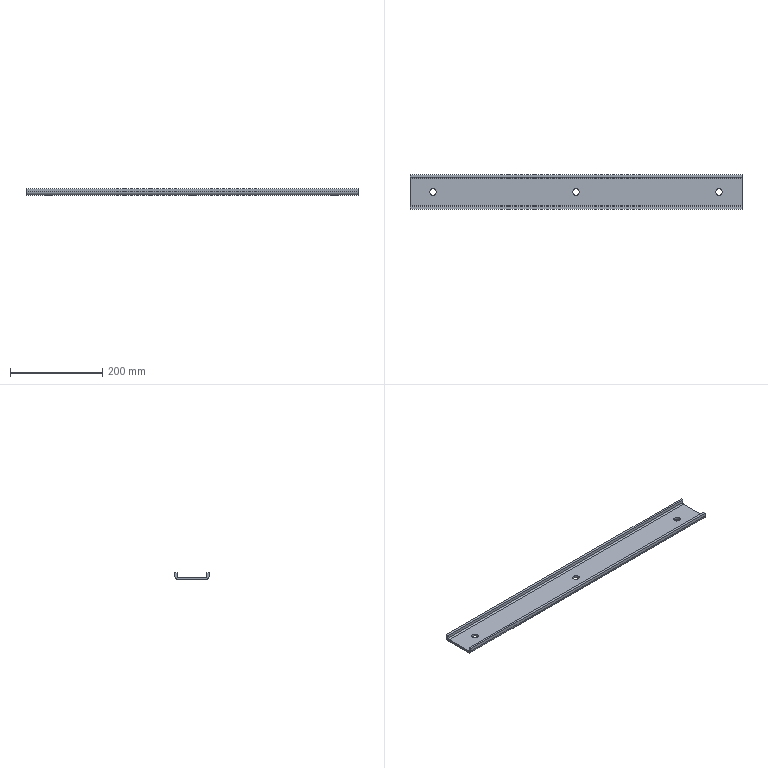Part | SolidWorks | features MoveFace 4, Fillet 2, BaseBody 1, ICE 1 | 1 solid | 20 faces | box 720 x 75 x 15 mm | volume 322694 mm3 | cylinder 10 | plane 10 | commonest cylinder face diameters 14 x6 6 x2 16 x2
STEP:
#1=CARTESIAN_POINT('',(-7.,0.,0.));
#2=VERTEX_POINT('',#1);
#3=CARTESIAN_POINT('',(7.,0.,0.));
#4=VERTEX_POINT('',#3);
#5=CARTESIAN_POINT('',(0.,0.,0.));
#6=DIRECTION('',(0.,0.,1.));
#7=DIRECTION('',(1.,0.,0.));
#8=AXIS2_PLACEMENT_3D('',#5,#6,#7);
#9=CIRCLE('',#8,7.);
#10=EDGE_CURVE('',#2,#4,#9,.T.);
#11=ORIENTED_EDGE('',*,*,#10,.F.);
#12=CARTESIAN_POINT('',(-7.,0.,5.));
#13=VERTEX_POINT('',#12);
#14=CARTESIAN_POINT('',(-7.,0.,-5.));
#15=DIRECTION('',(0.,0.,1.));
#16=VECTOR('',#15,1000.);
#17=LINE('',#14,#16);
#18=EDGE_CURVE('',#2,#13,#17,.T.);
#19=ORIENTED_EDGE('',*,*,#18,.T.);
#20=CARTESIAN_POINT('',(7.,0.,5.));
#21=VERTEX_POINT('',#20);
#22=CARTESIAN_POINT('',(0.,0.,5.));
#23=DIRECTION('',(0.,0.,-1.));
#24=DIRECTION('',(1.,0.,0.));
#25=AXIS2_PLACEMENT_3D('',#22,#23,#24);
#26=CIRCLE('',#25,7.);
#27=EDGE_CURVE('',#21,#13,#26,.T.);
#28=ORIENTED_EDGE('',*,*,#27,.F.);
#29=CARTESIAN_POINT('',(7.,0.,-5.));
#30=DIRECTION('',(0.,0.,1.));
#31=VECTOR('',#30,1000.);
#32=LINE('',#29,#31);
#33=EDGE_CURVE('',#4,#21,#32,.T.);
#34=ORIENTED_EDGE('',*,*,#33,.F.);
#35=EDGE_LOOP('',(#11,#19,#28,#34));
#36=FACE_OUTER_BOUND('',#35,.T.);
#37=CARTESIAN_POINT('',(0.,0.,-5.));
#38=DIRECTION('',(0.,0.,1.));
#39=DIRECTION('',(1.,0.,0.));
#40=AXIS2_PLACEMENT_3D('',#37,#38,#39);
#41=CYLINDRICAL_SURFACE('',#40,7.);
#42=ADVANCED_FACE('',(#36),#41,.F.);
#43=CARTESIAN_POINT('',(-317.,0.,0.));
#44=VERTEX_POINT('',#43);
#45=CARTESIAN_POINT('',(-303.,0.,0.));
#46=VERTEX_POINT('',#45);
#47=CARTESIAN_POINT('',(-310.,0.,0.));
#48=DIRECTION('',(0.,0.,1.));
#49=DIRECTION('',(1.,0.,0.));
#50=AXIS2_PLACEMENT_3D('',#47,#48,#49);
#51=CIRCLE('',#50,7.);
#52=EDGE_CURVE('',#44,#46,#51,.T.);
#53=ORIENTED_EDGE('',*,*,#52,.F.);
#54=CARTESIAN_POINT('',(-317.,0.,5.));
#55=VERTEX_POINT('',#54);
#56=CARTESIAN_POINT('',(-317.,0.,-5.));
#57=DIRECTION('',(0.,0.,1.));
#58=VECTOR('',#57,1000.);
#59=LINE('',#56,#58);
#60=EDGE_CURVE('',#44,#55,#59,.T.);
#61=ORIENTED_EDGE('',*,*,#60,.T.);
#62=CARTESIAN_POINT('',(-303.,0.,5.));
#63=VERTEX_POINT('',#62);
#64=CARTESIAN_POINT('',(-310.,0.,5.));
#65=DIRECTION('',(0.,0.,-1.));
#66=DIRECTION('',(1.,0.,0.));
#67=AXIS2_PLACEMENT_3D('',#64,#65,#66);
#68=CIRCLE('',#67,7.);
#69=EDGE_CURVE('',#63,#55,#68,.T.);
#70=ORIENTED_EDGE('',*,*,#69,.F.);
#71=CARTESIAN_POINT('',(-303.,0.,-5.));
#72=DIRECTION('',(0.,0.,1.));
#73=VECTOR('',#72,1000.);
#74=LINE('',#71,#73);
#75=EDGE_CURVE('',#46,#63,#74,.T.);
#76=ORIENTED_EDGE('',*,*,#75,.F.);
#77=EDGE_LOOP('',(#53,#61,#70,#76));
#78=FACE_OUTER_BOUND('',#77,.T.);
#79=CARTESIAN_POINT('',(-310.,0.,-5.));
#80=DIRECTION('',(0.,0.,1.));
#81=DIRECTION('',(1.,0.,0.));
#82=AXIS2_PLACEMENT_3D('',#79,#80,#81);
#83=CYLINDRICAL_SURFACE('',#82,7.);
#84=ADVANCED_FACE('',(#78),#83,.F.);
#85=CARTESIAN_POINT('',(303.,0.,0.));
#86=VERTEX_POINT('',#85);
#87=CARTESIAN_POINT('',(317.,0.,0.));
#88=VERTEX_POINT('',#87);
#89=CARTESIAN_POINT('',(310.,0.,0.));
#90=DIRECTION('',(0.,0.,1.));
#91=DIRECTION('',(1.,0.,0.));
#92=AXIS2_PLACEMENT_3D('',#89,#90,#91);
#93=CIRCLE('',#92,7.);
#94=EDGE_CURVE('',#86,#88,#93,.T.);
#95=ORIENTED_EDGE('',*,*,#94,.F.);
#96=CARTESIAN_POINT('',(303.,0.,5.));
#97=VERTEX_POINT('',#96);
#98=CARTESIAN_POINT('',(303.,0.,-5.));
#99=DIRECTION('',(0.,0.,1.));
#100=VECTOR('',#99,1000.);
#101=LINE('',#98,#100);
#102=EDGE_CURVE('',#86,#97,#101,.T.);
#103=ORIENTED_EDGE('',*,*,#102,.T.);
#104=CARTESIAN_POINT('',(317.,0.,5.));
#105=VERTEX_POINT('',#104);
#106=CARTESIAN_POINT('',(310.,0.,5.));
#107=DIRECTION('',(0.,0.,-1.));
#108=DIRECTION('',(1.,0.,0.));
#109=AXIS2_PLACEMENT_3D('',#106,#107,#108);
#110=CIRCLE('',#109,7.);
#111=EDGE_CURVE('',#105,#97,#110,.T.);
#112=ORIENTED_EDGE('',*,*,#111,.F.);
#113=CARTESIAN_POINT('',(317.,0.,-5.));
#114=DIRECTION('',(0.,0.,1.));
#115=VECTOR('',#114,1000.);
#116=LINE('',#113,#115);
#117=EDGE_CURVE('',#88,#105,#116,.T.);
#118=ORIENTED_EDGE('',*,*,#117,.F.);
#119=EDGE_LOOP('',(#95,#103,#112,#118));
#120=FACE_OUTER_BOUND('',#119,.T.);
#121=CARTESIAN_POINT('',(310.,0.,-5.));
#122=DIRECTION('',(0.,0.,1.));
#123=DIRECTION('',(1.,0.,0.));
#124=AXIS2_PLACEMENT_3D('',#121,#122,#123);
#125=CYLINDRICAL_SURFACE('',#124,7.);
#126=ADVANCED_FACE('',(#120),#125,.F.);
#127=ORIENTED_EDGE('',*,*,#27,.T.);
#128=CARTESIAN_POINT('',(0.,0.,5.));
#129=DIRECTION('',(0.,0.,-1.));
#130=DIRECTION('',(1.,0.,0.));
#131=AXIS2_PLACEMENT_3D('',#128,#129,#130);
#132=CIRCLE('',#131,7.);
#133=EDGE_CURVE('',#13,#21,#132,.T.);
#134=ORIENTED_EDGE('',*,*,#133,.T.);
#135=EDGE_LOOP('',(#127,#134));
#136=FACE_BOUND('',#135,.T.);
#137=ORIENTED_EDGE('',*,*,#69,.T.);
#138=CARTESIAN_POINT('',(-310.,0.,5.));
#139=DIRECTION('',(0.,0.,-1.));
#140=DIRECTION('',(1.,0.,0.));
#141=AXIS2_PLACEMENT_3D('',#138,#139,#140);
#142=CIRCLE('',#141,7.);
#143=EDGE_CURVE('',#55,#63,#142,.T.);
#144=ORIENTED_EDGE('',*,*,#143,.T.);
#145=EDGE_LOOP('',(#137,#144));
#146=FACE_BOUND('',#145,.T.);
#147=ORIENTED_EDGE('',*,*,#111,.T.);
#148=CARTESIAN_POINT('',(310.,0.,5.));
#149=DIRECTION('',(0.,0.,-1.));
#150=DIRECTION('',(1.,0.,0.));
#151=AXIS2_PLACEMENT_3D('',#148,#149,#150);
#152=CIRCLE('',#151,7.);
#153=EDGE_CURVE('',#97,#105,#152,.T.);
#154=ORIENTED_EDGE('',*,*,#153,.T.);
#155=EDGE_LOOP('',(#147,#154));
#156=FACE_BOUND('',#155,.T.);
#157=CARTESIAN_POINT('',(-360.,29.5,5.));
#158=VERTEX_POINT('',#157);
#159=CARTESIAN_POINT('',(-360.,-29.5,5.));
#160=VERTEX_POINT('',#159);
#161=CARTESIAN_POINT('',(-360.,0.,5.));
#162=DIRECTION('',(0.,-1.,0.));
#163=VECTOR('',#162,1000.);
#164=LINE('',#161,#163);
#165=EDGE_CURVE('',#158,#160,#164,.T.);
#166=ORIENTED_EDGE('',*,*,#165,.T.);
#167=CARTESIAN_POINT('',(360.,-29.5,5.));
#168=VERTEX_POINT('',#167);
#169=CARTESIAN_POINT('',(0.,-29.5,5.));
#170=DIRECTION('',(1.,0.,0.));
#171=VECTOR('',#170,1000.);
#172=LINE('',#169,#171);
#173=EDGE_CURVE('',#160,#168,#172,.T.);
#174=ORIENTED_EDGE('',*,*,#173,.T.);
#175=CARTESIAN_POINT('',(360.,29.5,5.));
#176=VERTEX_POINT('',#175);
#177=CARTESIAN_POINT('',(360.,0.,5.));
#178=DIRECTION('',(0.,1.,0.));
#179=VECTOR('',#178,1000.);
#180=LINE('',#177,#179);
#181=EDGE_CURVE('',#168,#176,#180,.T.);
#182=ORIENTED_EDGE('',*,*,#181,.T.);
#183=CARTESIAN_POINT('',(0.,29.5,5.));
#184=DIRECTION('',(-1.,0.,0.));
#185=VECTOR('',#184,1000.);
#186=LINE('',#183,#185);
#187=EDGE_CURVE('',#176,#158,#186,.T.);
#188=ORIENTED_EDGE('',*,*,#187,.T.);
#189=EDGE_LOOP('',(#166,#174,#182,#188));
#190=FACE_OUTER_BOUND('',#189,.T.);
#191=CARTESIAN_POINT('',(0.,0.,5.));
#192=DIRECTION('',(0.,0.,1.));
#193=DIRECTION('',(1.,0.,0.));
#194=AXIS2_PLACEMENT_3D('',#191,#192,#193);
#195=PLANE('',#194);
#196=ADVANCED_FACE('',(#136,#146,#156,#190),#195,.T.);
#197=CARTESIAN_POINT('',(-360.,-37.5,8.));
#198=VERTEX_POINT('',#197);
#199=CARTESIAN_POINT('',(-360.,-37.5,15.));
#200=VERTEX_POINT('',#199);
#201=CARTESIAN_POINT('',(-360.,-37.5,5.));
#202=DIRECTION('',(0.,0.,1.));
#203=VECTOR('',#202,1000.);
#204=LINE('',#201,#203);
#205=EDGE_CURVE('',#198,#200,#204,.T.);
#206=ORIENTED_EDGE('',*,*,#205,.F.);
#207=CARTESIAN_POINT('',(360.,-37.5,8.));
#208=VERTEX_POINT('',#207);
#209=CARTESIAN_POINT('',(-360.,-37.5,8.));
#210=DIRECTION('',(1.,0.,0.));
#211=VECTOR('',#210,1000.);
#212=LINE('',#209,#211);
#213=EDGE_CURVE('',#198,#208,#212,.T.);
#214=ORIENTED_EDGE('',*,*,#213,.T.);
#215=CARTESIAN_POINT('',(360.,-37.5,15.));
#216=VERTEX_POINT('',#215);
#217=CARTESIAN_POINT('',(360.,-37.5,5.));
#218=DIRECTION('',(0.,0.,-1.));
#219=VECTOR('',#218,1000.);
#220=LINE('',#217,#219);
#221=EDGE_CURVE('',#216,#208,#220,.T.);
#222=ORIENTED_EDGE('',*,*,#221,.F.);
#223=CARTESIAN_POINT('',(-300.,-37.5,15.));
#224=DIRECTION('',(1.,0.,0.));
#225=VECTOR('',#224,1000.);
#226=LINE('',#223,#225);
#227=EDGE_CURVE('',#200,#216,#226,.T.);
#228=ORIENTED_EDGE('',*,*,#227,.F.);
#229=EDGE_LOOP('',(#206,#214,#222,#228));
#230=FACE_OUTER_BOUND('',#229,.T.);
#231=CARTESIAN_POINT('',(-360.,-37.5,5.));
#232=DIRECTION('',(0.,1.,0.));
#233=DIRECTION('',(0.,0.,1.));
#234=AXIS2_PLACEMENT_3D('',#231,#232,#233);
#235=PLANE('',#234);
#236=ADVANCED_FACE('',(#230),#235,.F.);
#237=CARTESIAN_POINT('',(-360.,-29.5,0.));
#238=VERTEX_POINT('',#237);
#239=CARTESIAN_POINT('',(-360.,29.5,0.));
#240=VERTEX_POINT('',#239);
#241=CARTESIAN_POINT('',(-360.,37.5,0.));
#242=DIRECTION('',(0.,1.,0.));
#243=VECTOR('',#242,1000.);
#244=LINE('',#241,#243);
#245=EDGE_CURVE('',#238,#240,#244,.T.);
#246=ORIENTED_EDGE('',*,*,#245,.F.);
#247=CARTESIAN_POINT('',(-360.,-29.5,8.));
#248=DIRECTION('',(-1.,0.,0.));
#249=DIRECTION('',(0.,0.,-1.));
#250=AXIS2_PLACEMENT_3D('',#247,#248,#249);
#251=CIRCLE('',#250,8.);
#252=EDGE_CURVE('',#238,#198,#251,.T.);
#253=ORIENTED_EDGE('',*,*,#252,.T.);
#254=ORIENTED_EDGE('',*,*,#205,.T.);
#255=CARTESIAN_POINT('',(-360.,-32.5,15.));
#256=VERTEX_POINT('',#255);
#257=CARTESIAN_POINT('',(-360.,-37.5,15.));
#258=DIRECTION('',(0.,-1.,0.));
#259=VECTOR('',#258,1000.);
#260=LINE('',#257,#259);
#261=EDGE_CURVE('',#256,#200,#260,.T.);
#262=ORIENTED_EDGE('',*,*,#261,.F.);
#263=CARTESIAN_POINT('',(-360.,-32.5,8.));
#264=VERTEX_POINT('',#263);
#265=CARTESIAN_POINT('',(-360.,-32.5,15.));
#266=DIRECTION('',(0.,0.,-1.));
#267=VECTOR('',#266,1000.);
#268=LINE('',#265,#267);
#269=EDGE_CURVE('',#256,#264,#268,.T.);
#270=ORIENTED_EDGE('',*,*,#269,.T.);
#271=CARTESIAN_POINT('',(-360.,-29.5,8.));
#272=DIRECTION('',(1.,0.,0.));
#273=DIRECTION('',(0.,0.,-1.));
#274=AXIS2_PLACEMENT_3D('',#271,#272,#273);
#275=CIRCLE('',#274,3.);
#276=EDGE_CURVE('',#264,#160,#275,.T.);
#277=ORIENTED_EDGE('',*,*,#276,.T.);
#278=ORIENTED_EDGE('',*,*,#165,.F.);
#279=CARTESIAN_POINT('',(-360.,32.5,8.));
#280=VERTEX_POINT('',#279);
#281=CARTESIAN_POINT('',(-360.,29.5,8.));
#282=DIRECTION('',(1.,0.,0.));
#283=DIRECTION('',(0.,0.,-1.));
#284=AXIS2_PLACEMENT_3D('',#281,#282,#283);
#285=CIRCLE('',#284,3.);
#286=EDGE_CURVE('',#158,#280,#285,.T.);
#287=ORIENTED_EDGE('',*,*,#286,.T.);
#288=CARTESIAN_POINT('',(-360.,32.5,15.));
#289=VERTEX_POINT('',#288);
#290=CARTESIAN_POINT('',(-360.,32.5,15.));
#291=DIRECTION('',(0.,0.,-1.));
#292=VECTOR('',#291,1000.);
#293=LINE('',#290,#292);
#294=EDGE_CURVE('',#289,#280,#293,.T.);
#295=ORIENTED_EDGE('',*,*,#294,.F.);
#296=CARTESIAN_POINT('',(-360.,37.5,15.));
#297=VERTEX_POINT('',#296);
#298=CARTESIAN_POINT('',(-360.,37.5,15.));
#299=DIRECTION('',(0.,-1.,0.));
#300=VECTOR('',#299,1000.);
#301=LINE('',#298,#300);
#302=EDGE_CURVE('',#297,#289,#301,.T.);
#303=ORIENTED_EDGE('',*,*,#302,.F.);
#304=CARTESIAN_POINT('',(-360.,37.5,8.));
#305=VERTEX_POINT('',#304);
#306=CARTESIAN_POINT('',(-360.,37.5,5.));
#307=DIRECTION('',(0.,0.,1.));
#308=VECTOR('',#307,1000.);
#309=LINE('',#306,#308);
#310=EDGE_CURVE('',#305,#297,#309,.T.);
#311=ORIENTED_EDGE('',*,*,#310,.F.);
#312=CARTESIAN_POINT('',(-360.,29.5,8.));
#313=DIRECTION('',(-1.,0.,0.));
#314=DIRECTION('',(0.,0.,-1.));
#315=AXIS2_PLACEMENT_3D('',#312,#313,#314);
#316=CIRCLE('',#315,8.);
#317=EDGE_CURVE('',#305,#240,#316,.T.);
#318=ORIENTED_EDGE('',*,*,#317,.T.);
#319=EDGE_LOOP('',(#246,#253,#254,#262,#270,#277,#278,#287,#295,#303,#311,#318));
#320=FACE_OUTER_BOUND('',#319,.T.);
#321=CARTESIAN_POINT('',(-360.,37.5,5.));
#322=DIRECTION('',(1.,0.,0.));
#323=DIRECTION('',(0.,0.,-1.));
#324=AXIS2_PLACEMENT_3D('',#321,#322,#323);
#325=PLANE('',#324);
#326=ADVANCED_FACE('',(#320),#325,.F.);
#327=CARTESIAN_POINT('',(360.,37.5,8.));
#328=VERTEX_POINT('',#327);
#329=CARTESIAN_POINT('',(360.,37.5,15.));
#330=VERTEX_POINT('',#329);
#331=CARTESIAN_POINT('',(360.,37.5,5.));
#332=DIRECTION('',(0.,0.,1.));
#333=VECTOR('',#332,1000.);
#334=LINE('',#331,#333);
#335=EDGE_CURVE('',#328,#330,#334,.T.);
#336=ORIENTED_EDGE('',*,*,#335,.F.);
#337=CARTESIAN_POINT('',(-360.,37.5,8.));
#338=DIRECTION('',(-1.,0.,0.));
#339=VECTOR('',#338,1000.);
#340=LINE('',#337,#339);
#341=EDGE_CURVE('',#328,#305,#340,.T.);
#342=ORIENTED_EDGE('',*,*,#341,.T.);
#343=ORIENTED_EDGE('',*,*,#310,.T.);
#344=CARTESIAN_POINT('',(-300.,37.5,15.));
#345=DIRECTION('',(-1.,0.,0.));
#346=VECTOR('',#345,1000.);
#347=LINE('',#344,#346);
#348=EDGE_CURVE('',#330,#297,#347,.T.);
#349=ORIENTED_EDGE('',*,*,#348,.F.);
#350=EDGE_LOOP('',(#336,#342,#343,#349));
#351=FACE_OUTER_BOUND('',#350,.T.);
#352=CARTESIAN_POINT('',(-360.,37.5,5.));
#353=DIRECTION('',(0.,-1.,0.));
#354=DIRECTION('',(0.,0.,-1.));
#355=AXIS2_PLACEMENT_3D('',#352,#353,#354);
#356=PLANE('',#355);
#357=ADVANCED_FACE('',(#351),#356,.F.);
#358=ORIENTED_EDGE('',*,*,#221,.T.);
#359=CARTESIAN_POINT('',(360.,-29.5,0.));
#360=VERTEX_POINT('',#359);
#361=CARTESIAN_POINT('',(360.,-29.5,8.));
#362=DIRECTION('',(1.,0.,0.));
#363=DIRECTION('',(0.,0.,1.));
#364=AXIS2_PLACEMENT_3D('',#361,#362,#363);
#365=CIRCLE('',#364,8.);
#366=EDGE_CURVE('',#208,#360,#365,.T.);
#367=ORIENTED_EDGE('',*,*,#366,.T.);
#368=CARTESIAN_POINT('',(360.,29.5,0.));
#369=VERTEX_POINT('',#368);
#370=CARTESIAN_POINT('',(360.,37.5,0.));
#371=DIRECTION('',(0.,-1.,0.));
#372=VECTOR('',#371,1000.);
#373=LINE('',#370,#372);
#374=EDGE_CURVE('',#369,#360,#373,.T.);
#375=ORIENTED_EDGE('',*,*,#374,.F.);
#376=CARTESIAN_POINT('',(360.,29.5,8.));
#377=DIRECTION('',(1.,0.,0.));
#378=DIRECTION('',(0.,0.,1.));
#379=AXIS2_PLACEMENT_3D('',#376,#377,#378);
#380=CIRCLE('',#379,8.);
#381=EDGE_CURVE('',#369,#328,#380,.T.);
#382=ORIENTED_EDGE('',*,*,#381,.T.);
#383=ORIENTED_EDGE('',*,*,#335,.T.);
#384=CARTESIAN_POINT('',(360.,32.5,15.));
#385=VERTEX_POINT('',#384);
#386=CARTESIAN_POINT('',(360.,37.5,15.));
#387=DIRECTION('',(0.,1.,0.));
#388=VECTOR('',#387,1000.);
#389=LINE('',#386,#388);
#390=EDGE_CURVE('',#385,#330,#389,.T.);
#391=ORIENTED_EDGE('',*,*,#390,.F.);
#392=CARTESIAN_POINT('',(360.,32.5,8.));
#393=VERTEX_POINT('',#392);
#394=CARTESIAN_POINT('',(360.,32.5,15.));
#395=DIRECTION('',(0.,0.,-1.));
#396=VECTOR('',#395,1000.);
#397=LINE('',#394,#396);
#398=EDGE_CURVE('',#385,#393,#397,.T.);
#399=ORIENTED_EDGE('',*,*,#398,.T.);
#400=CARTESIAN_POINT('',(360.,29.5,8.));
#401=DIRECTION('',(-1.,0.,0.));
#402=DIRECTION('',(0.,0.,1.));
#403=AXIS2_PLACEMENT_3D('',#400,#401,#402);
#404=CIRCLE('',#403,3.);
#405=EDGE_CURVE('',#393,#176,#404,.T.);
#406=ORIENTED_EDGE('',*,*,#405,.T.);
#407=ORIENTED_EDGE('',*,*,#181,.F.);
#408=CARTESIAN_POINT('',(360.,-32.5,8.));
#409=VERTEX_POINT('',#408);
#410=CARTESIAN_POINT('',(360.,-29.5,8.));
#411=DIRECTION('',(-1.,0.,0.));
#412=DIRECTION('',(0.,0.,1.));
#413=AXIS2_PLACEMENT_3D('',#410,#411,#412);
#414=CIRCLE('',#413,3.);
#415=EDGE_CURVE('',#168,#409,#414,.T.);
#416=ORIENTED_EDGE('',*,*,#415,.T.);
#417=CARTESIAN_POINT('',(360.,-32.5,15.));
#418=VERTEX_POINT('',#417);
#419=CARTESIAN_POINT('',(360.,-32.5,15.));
#420=DIRECTION('',(0.,0.,-1.));
#421=VECTOR('',#420,1000.);
#422=LINE('',#419,#421);
#423=EDGE_CURVE('',#418,#409,#422,.T.);
#424=ORIENTED_EDGE('',*,*,#423,.F.);
#425=CARTESIAN_POINT('',(360.,-37.5,15.));
#426=DIRECTION('',(0.,1.,0.));
#427=VECTOR('',#426,1000.);
#428=LINE('',#425,#427);
#429=EDGE_CURVE('',#216,#418,#428,.T.);
#430=ORIENTED_EDGE('',*,*,#429,.F.);
#431=EDGE_LOOP('',(#358,#367,#375,#382,#383,#391,#399,#406,#407,#416,#424,#430));
#432=FACE_OUTER_BOUND('',#431,.T.);
#433=CARTESIAN_POINT('',(360.,37.5,5.));
#434=DIRECTION('',(-1.,0.,0.));
#435=DIRECTION('',(0.,0.,1.));
#436=AXIS2_PLACEMENT_3D('',#433,#434,#435);
#437=PLANE('',#436);
#438=ADVANCED_FACE('',(#432),#437,.F.);
#439=ORIENTED_EDGE('',*,*,#18,.F.);
#440=CARTESIAN_POINT('',(0.,0.,0.));
#441=DIRECTION('',(0.,0.,1.));
#442=DIRECTION('',(1.,0.,0.));
#443=AXIS2_PLACEMENT_3D('',#440,#441,#442);
#444=CIRCLE('',#443,7.);
#445=EDGE_CURVE('',#4,#2,#444,.T.);
#446=ORIENTED_EDGE('',*,*,#445,.F.);
#447=ORIENTED_EDGE('',*,*,#33,.T.);
#448=ORIENTED_EDGE('',*,*,#133,.F.);
#449=EDGE_LOOP('',(#439,#446,#447,#448));
#450=FACE_OUTER_BOUND('',#449,.T.);
#451=CARTESIAN_POINT('',(0.,0.,-5.));
#452=DIRECTION('',(0.,0.,1.));
#453=DIRECTION('',(1.,0.,0.));
#454=AXIS2_PLACEMENT_3D('',#451,#452,#453);
#455=CYLINDRICAL_SURFACE('',#454,7.);
#456=ADVANCED_FACE('',(#450),#455,.F.);
#457=ORIENTED_EDGE('',*,*,#60,.F.);
#458=CARTESIAN_POINT('',(-310.,0.,0.));
#459=DIRECTION('',(0.,0.,1.));
#460=DIRECTION('',(1.,0.,0.));
#461=AXIS2_PLACEMENT_3D('',#458,#459,#460);
#462=CIRCLE('',#461,7.);
#463=EDGE_CURVE('',#46,#44,#462,.T.);
#464=ORIENTED_EDGE('',*,*,#463,.F.);
#465=ORIENTED_EDGE('',*,*,#75,.T.);
#466=ORIENTED_EDGE('',*,*,#143,.F.);
#467=EDGE_LOOP('',(#457,#464,#465,#466));
#468=FACE_OUTER_BOUND('',#467,.T.);
#469=CARTESIAN_POINT('',(-310.,0.,-5.));
#470=DIRECTION('',(0.,0.,1.));
#471=DIRECTION('',(1.,0.,0.));
#472=AXIS2_PLACEMENT_3D('',#469,#470,#471);
#473=CYLINDRICAL_SURFACE('',#472,7.);
#474=ADVANCED_FACE('',(#468),#473,.F.);
#475=ORIENTED_EDGE('',*,*,#102,.F.);
#476=CARTESIAN_POINT('',(310.,0.,0.));
#477=DIRECTION('',(0.,0.,1.));
#478=DIRECTION('',(1.,0.,0.));
#479=AXIS2_PLACEMENT_3D('',#476,#477,#478);
#480=CIRCLE('',#479,7.);
#481=EDGE_CURVE('',#88,#86,#480,.T.);
#482=ORIENTED_EDGE('',*,*,#481,.F.);
#483=ORIENTED_EDGE('',*,*,#117,.T.);
#484=ORIENTED_EDGE('',*,*,#153,.F.);
#485=EDGE_LOOP('',(#475,#482,#483,#484));
#486=FACE_OUTER_BOUND('',#485,.T.);
#487=CARTESIAN_POINT('',(310.,0.,-5.));
#488=DIRECTION('',(0.,0.,1.));
#489=DIRECTION('',(1.,0.,0.));
#490=AXIS2_PLACEMENT_3D('',#487,#488,#489);
#491=CYLINDRICAL_SURFACE('',#490,7.);
#492=ADVANCED_FACE('',(#486),#491,.F.);
#493=ORIENTED_EDGE('',*,*,#374,.T.);
#494=CARTESIAN_POINT('',(0.,-29.5,0.));
#495=DIRECTION('',(-1.,0.,0.));
#496=VECTOR('',#495,1000.);
#497=LINE('',#494,#496);
#498=EDGE_CURVE('',#360,#238,#497,.T.);
#499=ORIENTED_EDGE('',*,*,#498,.T.);
#500=ORIENTED_EDGE('',*,*,#245,.T.);
#501=CARTESIAN_POINT('',(0.,29.5,0.));
#502=DIRECTION('',(1.,0.,0.));
#503=VECTOR('',#502,1000.);
#504=LINE('',#501,#503);
#505=EDGE_CURVE('',#240,#369,#504,.T.);
#506=ORIENTED_EDGE('',*,*,#505,.T.);
#507=EDGE_LOOP('',(#493,#499,#500,#506));
#508=FACE_OUTER_BOUND('',#507,.T.);
#509=ORIENTED_EDGE('',*,*,#445,.T.);
#510=ORIENTED_EDGE('',*,*,#10,.T.);
#511=EDGE_LOOP('',(#509,#510));
#512=FACE_BOUND('',#511,.T.);
#513=ORIENTED_EDGE('',*,*,#463,.T.);
#514=ORIENTED_EDGE('',*,*,#52,.T.);
#515=EDGE_LOOP('',(#513,#514));
#516=FACE_BOUND('',#515,.T.);
#517=ORIENTED_EDGE('',*,*,#481,.T.);
#518=ORIENTED_EDGE('',*,*,#94,.T.);
#519=EDGE_LOOP('',(#517,#518));
#520=FACE_BOUND('',#519,.T.);
#521=CARTESIAN_POINT('',(0.,0.,0.));
#522=DIRECTION('',(0.,0.,1.));
#523=DIRECTION('',(1.,0.,0.));
#524=AXIS2_PLACEMENT_3D('',#521,#522,#523);
#525=PLANE('',#524);
#526=ADVANCED_FACE('',(#508,#512,#516,#520),#525,.F.);
#527=ORIENTED_EDGE('',*,*,#294,.T.);
#528=CARTESIAN_POINT('',(-300.,32.5,8.));
#529=DIRECTION('',(1.,0.,0.));
#530=VECTOR('',#529,1000.);
#531=LINE('',#528,#530);
#532=EDGE_CURVE('',#280,#393,#531,.T.);
#533=ORIENTED_EDGE('',*,*,#532,.T.);
#534=ORIENTED_EDGE('',*,*,#398,.F.);
#535=CARTESIAN_POINT('',(-300.,32.5,15.));
#536=DIRECTION('',(1.,0.,0.));
#537=VECTOR('',#536,1000.);
#538=LINE('',#535,#537);
#539=EDGE_CURVE('',#289,#385,#538,.T.);
#540=ORIENTED_EDGE('',*,*,#539,.F.);
#541=EDGE_LOOP('',(#527,#533,#534,#540));
#542=FACE_OUTER_BOUND('',#541,.T.);
#543=CARTESIAN_POINT('',(-300.,32.5,15.));
#544=DIRECTION('',(0.,1.,0.));
#545=DIRECTION('',(-1.,0.,0.));
#546=AXIS2_PLACEMENT_3D('',#543,#544,#545);
#547=PLANE('',#546);
#548=ADVANCED_FACE('',(#542),#547,.F.);
#549=ORIENTED_EDGE('',*,*,#302,.T.);
#550=ORIENTED_EDGE('',*,*,#539,.T.);
#551=ORIENTED_EDGE('',*,*,#390,.T.);
#552=ORIENTED_EDGE('',*,*,#348,.T.);
#553=EDGE_LOOP('',(#549,#550,#551,#552));
#554=FACE_OUTER_BOUND('',#553,.T.);
#555=CARTESIAN_POINT('',(0.,0.,15.));
#556=DIRECTION('',(0.,0.,1.));
#557=DIRECTION('',(1.,0.,0.));
#558=AXIS2_PLACEMENT_3D('',#555,#556,#557);
#559=PLANE('',#558);
#560=ADVANCED_FACE('',(#554),#559,.T.);
#561=ORIENTED_EDGE('',*,*,#423,.T.);
#562=CARTESIAN_POINT('',(-300.,-32.5,8.));
#563=DIRECTION('',(-1.,0.,0.));
#564=VECTOR('',#563,1000.);
#565=LINE('',#562,#564);
#566=EDGE_CURVE('',#409,#264,#565,.T.);
#567=ORIENTED_EDGE('',*,*,#566,.T.);
#568=ORIENTED_EDGE('',*,*,#269,.F.);
#569=CARTESIAN_POINT('',(-300.,-32.5,15.));
#570=DIRECTION('',(-1.,0.,0.));
#571=VECTOR('',#570,1000.);
#572=LINE('',#569,#571);
#573=EDGE_CURVE('',#418,#256,#572,.T.);
#574=ORIENTED_EDGE('',*,*,#573,.F.);
#575=EDGE_LOOP('',(#561,#567,#568,#574));
#576=FACE_OUTER_BOUND('',#575,.T.);
#577=CARTESIAN_POINT('',(-300.,-32.5,15.));
#578=DIRECTION('',(0.,-1.,0.));
#579=DIRECTION('',(0.,0.,-1.));
#580=AXIS2_PLACEMENT_3D('',#577,#578,#579);
#581=PLANE('',#580);
#582=ADVANCED_FACE('',(#576),#581,.F.);
#583=ORIENTED_EDGE('',*,*,#261,.T.);
#584=ORIENTED_EDGE('',*,*,#227,.T.);
#585=ORIENTED_EDGE('',*,*,#429,.T.);
#586=ORIENTED_EDGE('',*,*,#573,.T.);
#587=EDGE_LOOP('',(#583,#584,#585,#586));
#588=FACE_OUTER_BOUND('',#587,.T.);
#589=CARTESIAN_POINT('',(0.,0.,15.));
#590=DIRECTION('',(0.,0.,-1.));
#591=DIRECTION('',(-1.,0.,0.));
#592=AXIS2_PLACEMENT_3D('',#589,#590,#591);
#593=PLANE('',#592);
#594=ADVANCED_FACE('',(#588),#593,.F.);
#595=ORIENTED_EDGE('',*,*,#366,.F.);
#596=ORIENTED_EDGE('',*,*,#213,.F.);
#597=ORIENTED_EDGE('',*,*,#252,.F.);
#598=ORIENTED_EDGE('',*,*,#498,.F.);
#599=EDGE_LOOP('',(#595,#596,#597,#598));
#600=FACE_OUTER_BOUND('',#599,.T.);
#601=CARTESIAN_POINT('',(0.,-29.5,8.));
#602=DIRECTION('',(-1.,0.,0.));
#603=DIRECTION('',(0.,0.,1.));
#604=AXIS2_PLACEMENT_3D('',#601,#602,#603);
#605=CYLINDRICAL_SURFACE('',#604,8.);
#606=ADVANCED_FACE('',(#600),#605,.T.);
#607=ORIENTED_EDGE('',*,*,#317,.F.);
#608=ORIENTED_EDGE('',*,*,#341,.F.);
#609=ORIENTED_EDGE('',*,*,#381,.F.);
#610=ORIENTED_EDGE('',*,*,#505,.F.);
#611=EDGE_LOOP('',(#607,#608,#609,#610));
#612=FACE_OUTER_BOUND('',#611,.T.);
#613=CARTESIAN_POINT('',(0.,29.5,8.));
#614=DIRECTION('',(1.,0.,0.));
#615=DIRECTION('',(0.,0.,-1.));
#616=AXIS2_PLACEMENT_3D('',#613,#614,#615);
#617=CYLINDRICAL_SURFACE('',#616,8.);
#618=ADVANCED_FACE('',(#612),#617,.T.);
#619=ORIENTED_EDGE('',*,*,#415,.F.);
#620=ORIENTED_EDGE('',*,*,#173,.F.);
#621=ORIENTED_EDGE('',*,*,#276,.F.);
#622=ORIENTED_EDGE('',*,*,#566,.F.);
#623=EDGE_LOOP('',(#619,#620,#621,#622));
#624=FACE_OUTER_BOUND('',#623,.T.);
#625=CARTESIAN_POINT('',(-300.,-29.5,8.));
#626=DIRECTION('',(-1.,0.,0.));
#627=DIRECTION('',(0.,0.,1.));
#628=AXIS2_PLACEMENT_3D('',#625,#626,#627);
#629=CYLINDRICAL_SURFACE('',#628,3.);
#630=ADVANCED_FACE('',(#624),#629,.F.);
#631=ORIENTED_EDGE('',*,*,#286,.F.);
#632=ORIENTED_EDGE('',*,*,#187,.F.);
#633=ORIENTED_EDGE('',*,*,#405,.F.);
#634=ORIENTED_EDGE('',*,*,#532,.F.);
#635=EDGE_LOOP('',(#631,#632,#633,#634));
#636=FACE_OUTER_BOUND('',#635,.T.);
#637=CARTESIAN_POINT('',(-300.,29.5,8.));
#638=DIRECTION('',(1.,0.,0.));
#639=DIRECTION('',(0.,1.,0.));
#640=AXIS2_PLACEMENT_3D('',#637,#638,#639);
#641=CYLINDRICAL_SURFACE('',#640,3.);
#642=ADVANCED_FACE('',(#636),#641,.F.);
#643=CLOSED_SHELL('',(#42,#84,#126,#196,#236,#326,#357,#438,#456,#474,#492,#526,#548,#560,#582,#594,#606,#618,#630,#642));
#644=MANIFOLD_SOLID_BREP('',#643);
#645=CARTESIAN_POINT('',(0.,0.,0.));
#646=DIRECTION('',(0.,0.,1.));
#647=DIRECTION('',(1.,0.,0.));
#648=AXIS2_PLACEMENT_3D('',#645,#646,#647);
#649=(LENGTH_UNIT()NAMED_UNIT(*)SI_UNIT(.MILLI.,.METRE.));
#650=UNCERTAINTY_MEASURE_WITH_UNIT(LENGTH_MEASURE(0.00001),#649,'','');
#651=(NAMED_UNIT(*)PLANE_ANGLE_UNIT()SI_UNIT($,.RADIAN.));
#652=(NAMED_UNIT(*)SI_UNIT($,.STERADIAN.)SOLID_ANGLE_UNIT());
#653=(GEOMETRIC_REPRESENTATION_CONTEXT(3)GLOBAL_UNCERTAINTY_ASSIGNED_CONTEXT((#650))GLOBAL_UNIT_ASSIGNED_CONTEXT((#649,#651,#652))REPRESENTATION_CONTEXT('',''));
#654=ADVANCED_BREP_SHAPE_REPRESENTATION('',(#644,#648),#653);